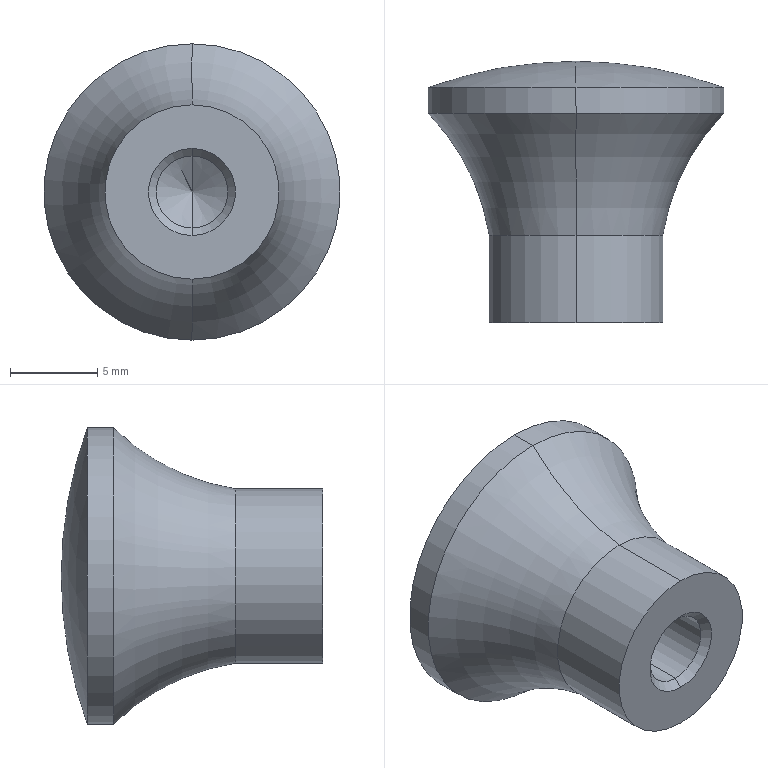Part | STEP file | HAQ07-M5^Air source cover plate | 1 solid | 15 faces | box 17 x 15 x 17 mm | volume 1673 mm3 | cylinder 6 | cone 4 | torus 2 | sphere 2 | plane 1 | commonest cylinder face diameters 4.134 x2 10 x2 17 x2
STEP:
#1=CARTESIAN_POINT('',(0.,0.,0.));
#2=DIRECTION('',(0.,0.,1.));
#3=DIRECTION('',(1.,0.,0.));
#4=AXIS2_PLACEMENT_3D('',#1,#2,#3);
#5=CARTESIAN_POINT('',(0.,18.75,-2.067));
#6=VERTEX_POINT('',#5);
#7=CARTESIAN_POINT('',(0.,18.75,2.067));
#8=VERTEX_POINT('',#7);
#9=CARTESIAN_POINT('',(0.,18.75,0.));
#10=DIRECTION('',(0.,1.,0.));
#11=DIRECTION('',(0.,0.,1.));
#12=AXIS2_PLACEMENT_3D('',#9,#10,#11);
#13=CIRCLE('',#12,2.067);
#14=CARTESIAN_POINT('',(0.,-480.057,0.));
#15=DIRECTION('',(0.,-1.,0.));
#16=DIRECTION('',(0.,0.,-1.));
#17=AXIS2_PLACEMENT_3D('',#14,#15,#16);
#18=CONICAL_SURFACE('',#17,866.025,1.047);
#19=CARTESIAN_POINT('',(9.425,-498.807));
#20=DIRECTION('',(-1.,0.));
#21=VECTOR('',#20,1.);
#22=LINE('',#19,#21);
#23=(GEOMETRIC_REPRESENTATION_CONTEXT(2)PARAMETRIC_REPRESENTATION_CONTEXT()REPRESENTATION_CONTEXT('',''));
#24=DEFINITIONAL_REPRESENTATION('',(#22),#23);
#25=PCURVE('',#18,#24);
#26=CARTESIAN_POINT('',(0.,19.943,0.));
#27=DIRECTION('',(0.,-1.,0.));
#28=DIRECTION('',(0.,0.,1.));
#29=AXIS2_PLACEMENT_3D('',#26,#27,#28);
#30=CYLINDRICAL_SURFACE('',#29,2.067);
#31=CARTESIAN_POINT('',(6.283,1.193));
#32=DIRECTION('',(-1.,0.));
#33=VECTOR('',#32,1.);
#34=LINE('',#31,#33);
#35=(GEOMETRIC_REPRESENTATION_CONTEXT(2)PARAMETRIC_REPRESENTATION_CONTEXT()REPRESENTATION_CONTEXT('',''));
#36=DEFINITIONAL_REPRESENTATION('',(#34),#35);
#37=PCURVE('',#30,#36);
#38=SURFACE_CURVE('',#13,(#25,#37),.PCURVE_S1.);
#39=EDGE_CURVE('',#6,#8,#38,.T.);
#40=ORIENTED_EDGE('',*,*,#39,.T.);
#41=CARTESIAN_POINT('',(0.,19.943,0.));
#42=VERTEX_POINT('',#41);
#43=CARTESIAN_POINT('',(0.,-480.057,866.025));
#44=DIRECTION('',(0.,-0.5,0.866));
#45=VECTOR('',#44,1.);
#46=LINE('',#43,#45);
#47=CARTESIAN_POINT('',(3.142,0.));
#48=DIRECTION('',(0.,1.));
#49=VECTOR('',#48,1.);
#50=LINE('',#47,#49);
#51=(GEOMETRIC_REPRESENTATION_CONTEXT(2)PARAMETRIC_REPRESENTATION_CONTEXT()REPRESENTATION_CONTEXT('',''));
#52=DEFINITIONAL_REPRESENTATION('',(#50),#51);
#53=PCURVE('',#18,#52);
#54=CARTESIAN_POINT('',(0.,-480.057,0.));
#55=DIRECTION('',(0.,-1.,0.));
#56=DIRECTION('',(0.,0.,-1.));
#57=AXIS2_PLACEMENT_3D('',#54,#55,#56);
#58=CONICAL_SURFACE('',#57,866.025,1.047);
#59=CARTESIAN_POINT('',(3.142,0.));
#60=DIRECTION('',(0.,1.));
#61=VECTOR('',#60,1.);
#62=LINE('',#59,#61);
#63=(GEOMETRIC_REPRESENTATION_CONTEXT(2)PARAMETRIC_REPRESENTATION_CONTEXT()REPRESENTATION_CONTEXT('',''));
#64=DEFINITIONAL_REPRESENTATION('',(#62),#63);
#65=PCURVE('',#58,#64);
#66=SURFACE_CURVE('',#46,(#53,#65),.PCURVE_S1.);
#67=EDGE_CURVE('',#42,#8,#66,.T.);
#68=ORIENTED_EDGE('',*,*,#67,.F.);
#69=CARTESIAN_POINT('',(0.,-480.057,-866.025));
#70=DIRECTION('',(0.,-0.5,-0.866));
#71=VECTOR('',#70,1.);
#72=LINE('',#69,#71);
#73=CARTESIAN_POINT('',(6.283,-500.));
#74=CARTESIAN_POINT('',(6.283,-499.982));
#75=CARTESIAN_POINT('',(6.283,-499.946));
#76=CARTESIAN_POINT('',(6.283,-499.892));
#77=CARTESIAN_POINT('',(6.283,-499.837));
#78=CARTESIAN_POINT('',(6.283,-499.783));
#79=CARTESIAN_POINT('',(6.283,-499.729));
#80=CARTESIAN_POINT('',(6.283,-499.675));
#81=CARTESIAN_POINT('',(6.283,-499.62));
#82=CARTESIAN_POINT('',(6.283,-499.566));
#83=CARTESIAN_POINT('',(6.283,-499.512));
#84=CARTESIAN_POINT('',(6.283,-499.458));
#85=CARTESIAN_POINT('',(6.283,-499.403));
#86=CARTESIAN_POINT('',(6.283,-499.349));
#87=CARTESIAN_POINT('',(6.283,-499.295));
#88=CARTESIAN_POINT('',(6.283,-499.241));
#89=CARTESIAN_POINT('',(6.283,-499.186));
#90=CARTESIAN_POINT('',(6.283,-499.132));
#91=CARTESIAN_POINT('',(6.283,-499.078));
#92=CARTESIAN_POINT('',(6.283,-499.024));
#93=CARTESIAN_POINT('',(6.283,-498.969));
#94=CARTESIAN_POINT('',(6.283,-498.915));
#95=CARTESIAN_POINT('',(6.283,-498.861));
#96=CARTESIAN_POINT('',(6.283,-498.825));
#97=CARTESIAN_POINT('',(6.283,-498.807));
#98=B_SPLINE_CURVE_WITH_KNOTS('',3,(#73,#74,#75,#76,#77,#78,#79,#80,#81,#82,#83,#84,#85,#86,#87,#88,#89,#90,#91,#92,#93,#94,#95,#96,#97),.UNSPECIFIED.,.F.,.F.,(4,1,1,1,1,1,1,1,1,1,1,1,1,1,1,1,1,1,1,1,1,1,4),(-1000.,-999.892,-999.783,-999.675,-999.566,-999.458,-999.349,-999.241,-999.132,-999.024,-998.915,-998.807,-998.698,-998.59,-998.481,-998.373,-998.264,-998.156,-998.047,-997.939,-997.83,-997.722,-997.613),.QUASI_UNIFORM_KNOTS.);
#99=(GEOMETRIC_REPRESENTATION_CONTEXT(2)PARAMETRIC_REPRESENTATION_CONTEXT()REPRESENTATION_CONTEXT('',''));
#100=DEFINITIONAL_REPRESENTATION('',(#98),#99);
#101=PCURVE('',#18,#100);
#102=CARTESIAN_POINT('',(0.,0.));
#103=DIRECTION('',(0.,1.));
#104=VECTOR('',#103,1.);
#105=LINE('',#102,#104);
#106=(GEOMETRIC_REPRESENTATION_CONTEXT(2)PARAMETRIC_REPRESENTATION_CONTEXT()REPRESENTATION_CONTEXT('',''));
#107=DEFINITIONAL_REPRESENTATION('',(#105),#106);
#108=PCURVE('',#58,#107);
#109=SURFACE_CURVE('',#72,(#101,#108),.PCURVE_S1.);
#110=EDGE_CURVE('',#42,#6,#109,.T.);
#111=ORIENTED_EDGE('',*,*,#110,.T.);
#112=EDGE_LOOP('',(#40,#68,#111));
#113=FACE_BOUND('',#112,.F.);
#114=ADVANCED_FACE('',(#113),#18,.F.);
#115=CARTESIAN_POINT('',(0.,10.433,2.067));
#116=VERTEX_POINT('',#115);
#117=CARTESIAN_POINT('',(0.,19.943,2.067));
#118=DIRECTION('',(0.,-1.,0.));
#119=VECTOR('',#118,1.);
#120=LINE('',#117,#119);
#121=CARTESIAN_POINT('',(0.,19.943,0.));
#122=DIRECTION('',(0.,-1.,0.));
#123=DIRECTION('',(0.,0.,1.));
#124=AXIS2_PLACEMENT_3D('',#121,#122,#123);
#125=CYLINDRICAL_SURFACE('',#124,2.067);
#126=CARTESIAN_POINT('',(6.283,0.));
#127=DIRECTION('',(0.,1.));
#128=VECTOR('',#127,1.);
#129=LINE('',#126,#128);
#130=(GEOMETRIC_REPRESENTATION_CONTEXT(2)PARAMETRIC_REPRESENTATION_CONTEXT()REPRESENTATION_CONTEXT('',''));
#131=DEFINITIONAL_REPRESENTATION('',(#129),#130);
#132=PCURVE('',#125,#131);
#133=CARTESIAN_POINT('',(0.,0.));
#134=DIRECTION('',(0.,1.));
#135=VECTOR('',#134,1.);
#136=LINE('',#133,#135);
#137=(GEOMETRIC_REPRESENTATION_CONTEXT(2)PARAMETRIC_REPRESENTATION_CONTEXT()REPRESENTATION_CONTEXT('',''));
#138=DEFINITIONAL_REPRESENTATION('',(#136),#137);
#139=PCURVE('',#30,#138);
#140=SURFACE_CURVE('',#120,(#132,#139),.PCURVE_S1.);
#141=EDGE_CURVE('',#8,#116,#140,.T.);
#142=ORIENTED_EDGE('',*,*,#141,.T.);
#143=CARTESIAN_POINT('',(0.,10.433,-2.067));
#144=VERTEX_POINT('',#143);
#145=CARTESIAN_POINT('',(0.,10.433,0.));
#146=DIRECTION('',(0.,1.,0.));
#147=DIRECTION('',(0.,0.,1.));
#148=AXIS2_PLACEMENT_3D('',#145,#146,#147);
#149=CIRCLE('',#148,2.067);
#150=CARTESIAN_POINT('',(6.283,9.51));
#151=DIRECTION('',(-1.,0.));
#152=VECTOR('',#151,1.);
#153=LINE('',#150,#152);
#154=(GEOMETRIC_REPRESENTATION_CONTEXT(2)PARAMETRIC_REPRESENTATION_CONTEXT()REPRESENTATION_CONTEXT('',''));
#155=DEFINITIONAL_REPRESENTATION('',(#153),#154);
#156=PCURVE('',#125,#155);
#157=CARTESIAN_POINT('',(0.,10.433,0.));
#158=DIRECTION('',(0.,-1.,0.));
#159=DIRECTION('',(0.,0.,-1.));
#160=AXIS2_PLACEMENT_3D('',#157,#158,#159);
#161=CONICAL_SURFACE('',#160,2.067,0.7854);
#162=CARTESIAN_POINT('',(3.142,0.));
#163=DIRECTION('',(-1.,0.));
#164=VECTOR('',#163,1.);
#165=LINE('',#162,#164);
#166=(GEOMETRIC_REPRESENTATION_CONTEXT(2)PARAMETRIC_REPRESENTATION_CONTEXT()REPRESENTATION_CONTEXT('',''));
#167=DEFINITIONAL_REPRESENTATION('',(#165),#166);
#168=PCURVE('',#161,#167);
#169=SURFACE_CURVE('',#149,(#156,#168),.PCURVE_S1.);
#170=EDGE_CURVE('',#116,#144,#169,.T.);
#171=ORIENTED_EDGE('',*,*,#170,.T.);
#172=CARTESIAN_POINT('',(0.,19.943,-2.067));
#173=DIRECTION('',(0.,-1.,0.));
#174=VECTOR('',#173,1.);
#175=LINE('',#172,#174);
#176=CARTESIAN_POINT('',(3.142,0.));
#177=DIRECTION('',(0.,1.));
#178=VECTOR('',#177,1.);
#179=LINE('',#176,#178);
#180=(GEOMETRIC_REPRESENTATION_CONTEXT(2)PARAMETRIC_REPRESENTATION_CONTEXT()REPRESENTATION_CONTEXT('',''));
#181=DEFINITIONAL_REPRESENTATION('',(#179),#180);
#182=PCURVE('',#125,#181);
#183=CARTESIAN_POINT('',(3.142,0.));
#184=DIRECTION('',(0.,1.));
#185=VECTOR('',#184,1.);
#186=LINE('',#183,#185);
#187=(GEOMETRIC_REPRESENTATION_CONTEXT(2)PARAMETRIC_REPRESENTATION_CONTEXT()REPRESENTATION_CONTEXT('',''));
#188=DEFINITIONAL_REPRESENTATION('',(#186),#187);
#189=PCURVE('',#30,#188);
#190=SURFACE_CURVE('',#175,(#182,#189),.PCURVE_S1.);
#191=EDGE_CURVE('',#6,#144,#190,.T.);
#192=ORIENTED_EDGE('',*,*,#191,.F.);
#193=CARTESIAN_POINT('',(0.,18.75,0.));
#194=DIRECTION('',(0.,1.,0.));
#195=DIRECTION('',(0.,0.,1.));
#196=AXIS2_PLACEMENT_3D('',#193,#194,#195);
#197=CIRCLE('',#196,2.067);
#198=CARTESIAN_POINT('',(6.283,1.193));
#199=DIRECTION('',(-1.,0.));
#200=VECTOR('',#199,1.);
#201=LINE('',#198,#200);
#202=(GEOMETRIC_REPRESENTATION_CONTEXT(2)PARAMETRIC_REPRESENTATION_CONTEXT()REPRESENTATION_CONTEXT('',''));
#203=DEFINITIONAL_REPRESENTATION('',(#201),#202);
#204=PCURVE('',#125,#203);
#205=CARTESIAN_POINT('',(3.142,-498.807));
#206=DIRECTION('',(-1.,0.));
#207=VECTOR('',#206,1.);
#208=LINE('',#205,#207);
#209=(GEOMETRIC_REPRESENTATION_CONTEXT(2)PARAMETRIC_REPRESENTATION_CONTEXT()REPRESENTATION_CONTEXT('',''));
#210=DEFINITIONAL_REPRESENTATION('',(#208),#209);
#211=PCURVE('',#58,#210);
#212=SURFACE_CURVE('',#197,(#204,#211),.PCURVE_S1.);
#213=EDGE_CURVE('',#8,#6,#212,.T.);
#214=ORIENTED_EDGE('',*,*,#213,.F.);
#215=EDGE_LOOP('',(#142,#171,#192,#214));
#216=FACE_BOUND('',#215,.F.);
#217=ADVANCED_FACE('',(#216),#125,.F.);
#218=CARTESIAN_POINT('',(0.,10.,-2.5));
#219=VERTEX_POINT('',#218);
#220=CARTESIAN_POINT('',(0.,10.433,-2.067));
#221=DIRECTION('',(0.,-0.7071,-0.7071));
#222=VECTOR('',#221,1.);
#223=LINE('',#220,#222);
#224=CARTESIAN_POINT('',(0.,10.433,0.));
#225=DIRECTION('',(0.,-1.,0.));
#226=DIRECTION('',(0.,0.,-1.));
#227=AXIS2_PLACEMENT_3D('',#224,#225,#226);
#228=CONICAL_SURFACE('',#227,2.067,0.7854);
#229=CARTESIAN_POINT('',(6.283,0.));
#230=DIRECTION('',(0.,1.));
#231=VECTOR('',#230,1.);
#232=LINE('',#229,#231);
#233=(GEOMETRIC_REPRESENTATION_CONTEXT(2)PARAMETRIC_REPRESENTATION_CONTEXT()REPRESENTATION_CONTEXT('',''));
#234=DEFINITIONAL_REPRESENTATION('',(#232),#233);
#235=PCURVE('',#228,#234);
#236=CARTESIAN_POINT('',(0.,0.));
#237=DIRECTION('',(0.,1.));
#238=VECTOR('',#237,1.);
#239=LINE('',#236,#238);
#240=(GEOMETRIC_REPRESENTATION_CONTEXT(2)PARAMETRIC_REPRESENTATION_CONTEXT()REPRESENTATION_CONTEXT('',''));
#241=DEFINITIONAL_REPRESENTATION('',(#239),#240);
#242=PCURVE('',#161,#241);
#243=SURFACE_CURVE('',#223,(#235,#242),.PCURVE_S1.);
#244=EDGE_CURVE('',#144,#219,#243,.T.);
#245=ORIENTED_EDGE('',*,*,#244,.T.);
#246=CARTESIAN_POINT('',(0.,10.,2.5));
#247=VERTEX_POINT('',#246);
#248=CARTESIAN_POINT('',(0.,10.,0.));
#249=DIRECTION('',(0.,1.,0.));
#250=DIRECTION('',(0.,0.,1.));
#251=AXIS2_PLACEMENT_3D('',#248,#249,#250);
#252=CIRCLE('',#251,2.5);
#253=CARTESIAN_POINT('',(9.425,0.433));
#254=DIRECTION('',(-1.,0.));
#255=VECTOR('',#254,1.);
#256=LINE('',#253,#255);
#257=(GEOMETRIC_REPRESENTATION_CONTEXT(2)PARAMETRIC_REPRESENTATION_CONTEXT()REPRESENTATION_CONTEXT('',''));
#258=DEFINITIONAL_REPRESENTATION('',(#256),#257);
#259=PCURVE('',#228,#258);
#260=CARTESIAN_POINT('',(0.,10.,2.5));
#261=DIRECTION('',(0.,1.,0.));
#262=DIRECTION('',(1.,0.,0.));
#263=AXIS2_PLACEMENT_3D('',#260,#261,#262);
#264=PLANE('',#263);
#265=CARTESIAN_POINT('',(0.,2.5));
#266=DIRECTION('',(0.,-1.));
#267=AXIS2_PLACEMENT_2D('',#265,#266);
#268=CIRCLE('',#267,2.5);
#269=(GEOMETRIC_REPRESENTATION_CONTEXT(2)PARAMETRIC_REPRESENTATION_CONTEXT()REPRESENTATION_CONTEXT('',''));
#270=DEFINITIONAL_REPRESENTATION('',(#268),#269);
#271=PCURVE('',#264,#270);
#272=SURFACE_CURVE('',#252,(#259,#271),.PCURVE_S1.);
#273=EDGE_CURVE('',#219,#247,#272,.T.);
#274=ORIENTED_EDGE('',*,*,#273,.T.);
#275=CARTESIAN_POINT('',(0.,10.433,2.067));
#276=DIRECTION('',(0.,-0.7071,0.7071));
#277=VECTOR('',#276,1.);
#278=LINE('',#275,#277);
#279=CARTESIAN_POINT('',(3.142,0.));
#280=DIRECTION('',(0.,1.));
#281=VECTOR('',#280,1.);
#282=LINE('',#279,#281);
#283=(GEOMETRIC_REPRESENTATION_CONTEXT(2)PARAMETRIC_REPRESENTATION_CONTEXT()REPRESENTATION_CONTEXT('',''));
#284=DEFINITIONAL_REPRESENTATION('',(#282),#283);
#285=PCURVE('',#228,#284);
#286=CARTESIAN_POINT('',(3.142,0.));
#287=DIRECTION('',(0.,1.));
#288=VECTOR('',#287,1.);
#289=LINE('',#286,#288);
#290=(GEOMETRIC_REPRESENTATION_CONTEXT(2)PARAMETRIC_REPRESENTATION_CONTEXT()REPRESENTATION_CONTEXT('',''));
#291=DEFINITIONAL_REPRESENTATION('',(#289),#290);
#292=PCURVE('',#161,#291);
#293=SURFACE_CURVE('',#278,(#285,#292),.PCURVE_S1.);
#294=EDGE_CURVE('',#116,#247,#293,.T.);
#295=ORIENTED_EDGE('',*,*,#294,.F.);
#296=CARTESIAN_POINT('',(0.,10.433,0.));
#297=DIRECTION('',(0.,1.,0.));
#298=DIRECTION('',(0.,0.,1.));
#299=AXIS2_PLACEMENT_3D('',#296,#297,#298);
#300=CIRCLE('',#299,2.067);
#301=CARTESIAN_POINT('',(9.425,0.));
#302=DIRECTION('',(-1.,0.));
#303=VECTOR('',#302,1.);
#304=LINE('',#301,#303);
#305=(GEOMETRIC_REPRESENTATION_CONTEXT(2)PARAMETRIC_REPRESENTATION_CONTEXT()REPRESENTATION_CONTEXT('',''));
#306=DEFINITIONAL_REPRESENTATION('',(#304),#305);
#307=PCURVE('',#228,#306);
#308=CARTESIAN_POINT('',(6.283,9.51));
#309=DIRECTION('',(-1.,0.));
#310=VECTOR('',#309,1.);
#311=LINE('',#308,#310);
#312=(GEOMETRIC_REPRESENTATION_CONTEXT(2)PARAMETRIC_REPRESENTATION_CONTEXT()REPRESENTATION_CONTEXT('',''));
#313=DEFINITIONAL_REPRESENTATION('',(#311),#312);
#314=PCURVE('',#30,#313);
#315=SURFACE_CURVE('',#300,(#307,#314),.PCURVE_S1.);
#316=EDGE_CURVE('',#144,#116,#315,.T.);
#317=ORIENTED_EDGE('',*,*,#316,.F.);
#318=EDGE_LOOP('',(#245,#274,#295,#317));
#319=FACE_BOUND('',#318,.F.);
#320=ADVANCED_FACE('',(#319),#228,.F.);
#321=CARTESIAN_POINT('',(0.,15.,-5.));
#322=VERTEX_POINT('',#321);
#323=CARTESIAN_POINT('',(0.,15.,5.));
#324=VERTEX_POINT('',#323);
#325=CARTESIAN_POINT('',(0.,15.,0.));
#326=DIRECTION('',(0.,1.,0.));
#327=DIRECTION('',(0.,0.,1.));
#328=AXIS2_PLACEMENT_3D('',#325,#326,#327);
#329=CIRCLE('',#328,5.);
#330=CARTESIAN_POINT('',(0.,19.943,0.));
#331=DIRECTION('',(0.,-1.,0.));
#332=DIRECTION('',(0.,0.,1.));
#333=AXIS2_PLACEMENT_3D('',#330,#331,#332);
#334=CYLINDRICAL_SURFACE('',#333,5.);
#335=CARTESIAN_POINT('',(6.283,4.943));
#336=DIRECTION('',(-1.,0.));
#337=VECTOR('',#336,1.);
#338=LINE('',#335,#337);
#339=(GEOMETRIC_REPRESENTATION_CONTEXT(2)PARAMETRIC_REPRESENTATION_CONTEXT()REPRESENTATION_CONTEXT('',''));
#340=DEFINITIONAL_REPRESENTATION('',(#338),#339);
#341=PCURVE('',#334,#340);
#342=CARTESIAN_POINT('',(0.,13.073,0.));
#343=DIRECTION('',(0.,1.,0.));
#344=DIRECTION('',(0.,0.,1.));
#345=AXIS2_PLACEMENT_3D('',#342,#343,#344);
#346=TOROIDAL_SURFACE('',#345,17.604,12.75);
#347=CARTESIAN_POINT('',(0.,2.99));
#348=DIRECTION('',(1.,0.));
#349=VECTOR('',#348,1.);
#350=LINE('',#347,#349);
#351=(GEOMETRIC_REPRESENTATION_CONTEXT(2)PARAMETRIC_REPRESENTATION_CONTEXT()REPRESENTATION_CONTEXT('',''));
#352=DEFINITIONAL_REPRESENTATION('',(#350),#351);
#353=PCURVE('',#346,#352);
#354=SURFACE_CURVE('',#329,(#341,#353),.PCURVE_S1.);
#355=EDGE_CURVE('',#322,#324,#354,.T.);
#356=ORIENTED_EDGE('',*,*,#355,.F.);
#357=CARTESIAN_POINT('',(0.,10.,-5.));
#358=VERTEX_POINT('',#357);
#359=CARTESIAN_POINT('',(0.,19.943,-5.));
#360=DIRECTION('',(0.,-1.,0.));
#361=VECTOR('',#360,1.);
#362=LINE('',#359,#361);
#363=CARTESIAN_POINT('',(3.142,0.));
#364=DIRECTION('',(0.,1.));
#365=VECTOR('',#364,1.);
#366=LINE('',#363,#365);
#367=(GEOMETRIC_REPRESENTATION_CONTEXT(2)PARAMETRIC_REPRESENTATION_CONTEXT()REPRESENTATION_CONTEXT('',''));
#368=DEFINITIONAL_REPRESENTATION('',(#366),#367);
#369=PCURVE('',#334,#368);
#370=CARTESIAN_POINT('',(0.,19.943,0.));
#371=DIRECTION('',(0.,-1.,0.));
#372=DIRECTION('',(0.,0.,1.));
#373=AXIS2_PLACEMENT_3D('',#370,#371,#372);
#374=CYLINDRICAL_SURFACE('',#373,5.);
#375=CARTESIAN_POINT('',(3.142,0.));
#376=DIRECTION('',(0.,1.));
#377=VECTOR('',#376,1.);
#378=LINE('',#375,#377);
#379=(GEOMETRIC_REPRESENTATION_CONTEXT(2)PARAMETRIC_REPRESENTATION_CONTEXT()REPRESENTATION_CONTEXT('',''));
#380=DEFINITIONAL_REPRESENTATION('',(#378),#379);
#381=PCURVE('',#374,#380);
#382=SURFACE_CURVE('',#362,(#369,#381),.PCURVE_S1.);
#383=EDGE_CURVE('',#322,#358,#382,.T.);
#384=ORIENTED_EDGE('',*,*,#383,.T.);
#385=CARTESIAN_POINT('',(0.,10.,5.));
#386=VERTEX_POINT('',#385);
#387=CARTESIAN_POINT('',(0.,10.,0.));
#388=DIRECTION('',(0.,1.,0.));
#389=DIRECTION('',(0.,0.,1.));
#390=AXIS2_PLACEMENT_3D('',#387,#388,#389);
#391=CIRCLE('',#390,5.);
#392=CARTESIAN_POINT('',(6.283,9.943));
#393=DIRECTION('',(-1.,0.));
#394=VECTOR('',#393,1.);
#395=LINE('',#392,#394);
#396=(GEOMETRIC_REPRESENTATION_CONTEXT(2)PARAMETRIC_REPRESENTATION_CONTEXT()REPRESENTATION_CONTEXT('',''));
#397=DEFINITIONAL_REPRESENTATION('',(#395),#396);
#398=PCURVE('',#334,#397);
#399=CARTESIAN_POINT('',(0.,2.5));
#400=DIRECTION('',(0.,-1.));
#401=AXIS2_PLACEMENT_2D('',#399,#400);
#402=CIRCLE('',#401,5.);
#403=(GEOMETRIC_REPRESENTATION_CONTEXT(2)PARAMETRIC_REPRESENTATION_CONTEXT()REPRESENTATION_CONTEXT('',''));
#404=DEFINITIONAL_REPRESENTATION('',(#402),#403);
#405=PCURVE('',#264,#404);
#406=SURFACE_CURVE('',#391,(#398,#405),.PCURVE_S1.);
#407=EDGE_CURVE('',#358,#386,#406,.T.);
#408=ORIENTED_EDGE('',*,*,#407,.T.);
#409=CARTESIAN_POINT('',(0.,19.943,5.));
#410=DIRECTION('',(0.,-1.,0.));
#411=VECTOR('',#410,1.);
#412=LINE('',#409,#411);
#413=CARTESIAN_POINT('',(0.,0.));
#414=DIRECTION('',(0.,1.));
#415=VECTOR('',#414,1.);
#416=LINE('',#413,#415);
#417=(GEOMETRIC_REPRESENTATION_CONTEXT(2)PARAMETRIC_REPRESENTATION_CONTEXT()REPRESENTATION_CONTEXT('',''));
#418=DEFINITIONAL_REPRESENTATION('',(#416),#417);
#419=PCURVE('',#334,#418);
#420=CARTESIAN_POINT('',(6.283,0.));
#421=DIRECTION('',(0.,1.));
#422=VECTOR('',#421,1.);
#423=LINE('',#420,#422);
#424=(GEOMETRIC_REPRESENTATION_CONTEXT(2)PARAMETRIC_REPRESENTATION_CONTEXT()REPRESENTATION_CONTEXT('',''));
#425=DEFINITIONAL_REPRESENTATION('',(#423),#424);
#426=PCURVE('',#374,#425);
#427=SURFACE_CURVE('',#412,(#419,#426),.PCURVE_S1.);
#428=EDGE_CURVE('',#324,#386,#427,.T.);
#429=ORIENTED_EDGE('',*,*,#428,.F.);
#430=EDGE_LOOP('',(#356,#384,#408,#429));
#431=FACE_BOUND('',#430,.T.);
#432=ADVANCED_FACE('',(#431),#334,.T.);
#433=CARTESIAN_POINT('',(0.,22.,8.5));
#434=VERTEX_POINT('',#433);
#435=CARTESIAN_POINT('',(0.,13.073,17.604));
#436=DIRECTION('',(-1.,0.,0.));
#437=DIRECTION('',(0.,-1.,0.));
#438=AXIS2_PLACEMENT_3D('',#435,#436,#437);
#439=CIRCLE('',#438,12.75);
#440=CARTESIAN_POINT('',(6.283,-1.571));
#441=DIRECTION('',(0.,1.));
#442=VECTOR('',#441,1.);
#443=LINE('',#440,#442);
#444=(GEOMETRIC_REPRESENTATION_CONTEXT(2)PARAMETRIC_REPRESENTATION_CONTEXT()REPRESENTATION_CONTEXT('',''));
#445=DEFINITIONAL_REPRESENTATION('',(#443),#444);
#446=PCURVE('',#346,#445);
#447=CARTESIAN_POINT('',(0.,13.073,0.));
#448=DIRECTION('',(0.,1.,0.));
#449=DIRECTION('',(0.,0.,1.));
#450=AXIS2_PLACEMENT_3D('',#447,#448,#449);
#451=TOROIDAL_SURFACE('',#450,17.604,12.75);
#452=CARTESIAN_POINT('',(0.,-1.571));
#453=DIRECTION('',(0.,1.));
#454=VECTOR('',#453,1.);
#455=LINE('',#452,#454);
#456=(GEOMETRIC_REPRESENTATION_CONTEXT(2)PARAMETRIC_REPRESENTATION_CONTEXT()REPRESENTATION_CONTEXT('',''));
#457=DEFINITIONAL_REPRESENTATION('',(#455),#456);
#458=PCURVE('',#451,#457);
#459=SURFACE_CURVE('',#439,(#446,#458),.PCURVE_S1.);
#460=EDGE_CURVE('',#434,#324,#459,.T.);
#461=ORIENTED_EDGE('',*,*,#460,.T.);
#462=ORIENTED_EDGE('',*,*,#355,.F.);
#463=CARTESIAN_POINT('',(0.,22.,-8.5));
#464=VERTEX_POINT('',#463);
#465=CARTESIAN_POINT('',(0.,13.073,-17.604));
#466=DIRECTION('',(1.,0.,0.));
#467=DIRECTION('',(0.,1.,0.));
#468=AXIS2_PLACEMENT_3D('',#465,#466,#467);
#469=CIRCLE('',#468,12.75);
#470=CARTESIAN_POINT('',(3.142,1.571));
#471=DIRECTION('',(0.,1.));
#472=VECTOR('',#471,1.);
#473=LINE('',#470,#472);
#474=(GEOMETRIC_REPRESENTATION_CONTEXT(2)PARAMETRIC_REPRESENTATION_CONTEXT()REPRESENTATION_CONTEXT('',''));
#475=DEFINITIONAL_REPRESENTATION('',(#473),#474);
#476=PCURVE('',#346,#475);
#477=CARTESIAN_POINT('',(3.142,1.571));
#478=DIRECTION('',(0.,1.));
#479=VECTOR('',#478,1.);
#480=LINE('',#477,#479);
#481=(GEOMETRIC_REPRESENTATION_CONTEXT(2)PARAMETRIC_REPRESENTATION_CONTEXT()REPRESENTATION_CONTEXT('',''));
#482=DEFINITIONAL_REPRESENTATION('',(#480),#481);
#483=PCURVE('',#451,#482);
#484=SURFACE_CURVE('',#469,(#476,#483),.PCURVE_S1.);
#485=EDGE_CURVE('',#464,#322,#484,.T.);
#486=ORIENTED_EDGE('',*,*,#485,.F.);
#487=CARTESIAN_POINT('',(0.,22.,0.));
#488=DIRECTION('',(0.,1.,0.));
#489=DIRECTION('',(0.,0.,1.));
#490=AXIS2_PLACEMENT_3D('',#487,#488,#489);
#491=CIRCLE('',#490,8.5);
#492=CARTESIAN_POINT('',(0.,2.366));
#493=DIRECTION('',(1.,0.));
#494=VECTOR('',#493,1.);
#495=LINE('',#492,#494);
#496=(GEOMETRIC_REPRESENTATION_CONTEXT(2)PARAMETRIC_REPRESENTATION_CONTEXT()REPRESENTATION_CONTEXT('',''));
#497=DEFINITIONAL_REPRESENTATION('',(#495),#496);
#498=PCURVE('',#346,#497);
#499=CARTESIAN_POINT('',(0.,19.943,0.));
#500=DIRECTION('',(0.,-1.,0.));
#501=DIRECTION('',(0.,0.,1.));
#502=AXIS2_PLACEMENT_3D('',#499,#500,#501);
#503=CYLINDRICAL_SURFACE('',#502,8.5);
#504=CARTESIAN_POINT('',(6.283,-2.057));
#505=DIRECTION('',(-1.,0.));
#506=VECTOR('',#505,1.);
#507=LINE('',#504,#506);
#508=(GEOMETRIC_REPRESENTATION_CONTEXT(2)PARAMETRIC_REPRESENTATION_CONTEXT()REPRESENTATION_CONTEXT('',''));
#509=DEFINITIONAL_REPRESENTATION('',(#507),#508);
#510=PCURVE('',#503,#509);
#511=SURFACE_CURVE('',#491,(#498,#510),.PCURVE_S1.);
#512=EDGE_CURVE('',#464,#434,#511,.T.);
#513=ORIENTED_EDGE('',*,*,#512,.T.);
#514=EDGE_LOOP('',(#461,#462,#486,#513));
#515=FACE_BOUND('',#514,.F.);
#516=ADVANCED_FACE('',(#515),#346,.F.);
#517=CARTESIAN_POINT('',(0.,23.5,-8.5));
#518=VERTEX_POINT('',#517);
#519=CARTESIAN_POINT('',(0.,23.5,8.5));
#520=VERTEX_POINT('',#519);
#521=CARTESIAN_POINT('',(0.,23.5,0.));
#522=DIRECTION('',(0.,1.,0.));
#523=DIRECTION('',(0.,0.,1.));
#524=AXIS2_PLACEMENT_3D('',#521,#522,#523);
#525=CIRCLE('',#524,8.5);
#526=CARTESIAN_POINT('',(6.283,-3.557));
#527=DIRECTION('',(-1.,0.));
#528=VECTOR('',#527,1.);
#529=LINE('',#526,#528);
#530=(GEOMETRIC_REPRESENTATION_CONTEXT(2)PARAMETRIC_REPRESENTATION_CONTEXT()REPRESENTATION_CONTEXT('',''));
#531=DEFINITIONAL_REPRESENTATION('',(#529),#530);
#532=PCURVE('',#503,#531);
#533=CARTESIAN_POINT('',(0.,0.1667,0.));
#534=DIRECTION('',(-1.,0.,0.));
#535=DIRECTION('',(0.,0.,-1.));
#536=AXIS2_PLACEMENT_3D('',#533,#534,#535);
#537=SPHERICAL_SURFACE('',#536,24.833);
#538=CARTESIAN_POINT('',(5.062,0.));
#539=CARTESIAN_POINT('',(5.062,0.01629));
#540=CARTESIAN_POINT('',(5.06,0.04888));
#541=CARTESIAN_POINT('',(5.05,0.09688));
#542=CARTESIAN_POINT('',(5.033,0.1431));
#543=CARTESIAN_POINT('',(5.011,0.1867));
#544=CARTESIAN_POINT('',(4.982,0.2268));
#545=CARTESIAN_POINT('',(4.947,0.2625));
#546=CARTESIAN_POINT('',(4.908,0.2931));
#547=CARTESIAN_POINT('',(4.863,0.3177));
#548=CARTESIAN_POINT('',(4.815,0.3358));
#549=CARTESIAN_POINT('',(4.764,0.3469));
#550=CARTESIAN_POINT('',(4.712,0.3506));
#551=CARTESIAN_POINT('',(4.66,0.3469));
#552=CARTESIAN_POINT('',(4.61,0.3358));
#553=CARTESIAN_POINT('',(4.562,0.3177));
#554=CARTESIAN_POINT('',(4.517,0.2931));
#555=CARTESIAN_POINT('',(4.477,0.2625));
#556=CARTESIAN_POINT('',(4.443,0.2268));
#557=CARTESIAN_POINT('',(4.414,0.1867));
#558=CARTESIAN_POINT('',(4.391,0.1431));
#559=CARTESIAN_POINT('',(4.375,0.09688));
#560=CARTESIAN_POINT('',(4.365,0.04888));
#561=CARTESIAN_POINT('',(4.363,0.01629));
#562=CARTESIAN_POINT('',(4.363,0.));
#563=B_SPLINE_CURVE_WITH_KNOTS('',3,(#538,#539,#540,#541,#542,#543,#544,#545,#546,#547,#548,#549,#550,#551,#552,#553,#554,#555,#556,#557,#558,#559,#560,#561,#562),.UNSPECIFIED.,.F.,.F.,(4,1,1,1,1,1,1,1,1,1,1,1,1,1,1,1,1,1,1,1,1,1,4),(3.142,3.284,3.427,3.57,3.713,3.856,3.998,4.141,4.284,4.427,4.57,4.712,4.855,4.998,5.141,5.284,5.426,5.569,5.712,5.855,5.998,6.14,6.283),.QUASI_UNIFORM_KNOTS.);
#564=(GEOMETRIC_REPRESENTATION_CONTEXT(2)PARAMETRIC_REPRESENTATION_CONTEXT()REPRESENTATION_CONTEXT('',''));
#565=DEFINITIONAL_REPRESENTATION('',(#563),#564);
#566=PCURVE('',#537,#565);
#567=SURFACE_CURVE('',#525,(#532,#566),.PCURVE_S1.);
#568=EDGE_CURVE('',#518,#520,#567,.T.);
#569=ORIENTED_EDGE('',*,*,#568,.F.);
#570=CARTESIAN_POINT('',(0.,19.943,-8.5));
#571=DIRECTION('',(0.,-1.,0.));
#572=VECTOR('',#571,1.);
#573=LINE('',#570,#572);
#574=CARTESIAN_POINT('',(3.142,0.));
#575=DIRECTION('',(0.,1.));
#576=VECTOR('',#575,1.);
#577=LINE('',#574,#576);
#578=(GEOMETRIC_REPRESENTATION_CONTEXT(2)PARAMETRIC_REPRESENTATION_CONTEXT()REPRESENTATION_CONTEXT('',''));
#579=DEFINITIONAL_REPRESENTATION('',(#577),#578);
#580=PCURVE('',#503,#579);
#581=CARTESIAN_POINT('',(0.,19.943,0.));
#582=DIRECTION('',(0.,-1.,0.));
#583=DIRECTION('',(0.,0.,1.));
#584=AXIS2_PLACEMENT_3D('',#581,#582,#583);
#585=CYLINDRICAL_SURFACE('',#584,8.5);
#586=CARTESIAN_POINT('',(3.142,0.));
#587=DIRECTION('',(0.,1.));
#588=VECTOR('',#587,1.);
#589=LINE('',#586,#588);
#590=(GEOMETRIC_REPRESENTATION_CONTEXT(2)PARAMETRIC_REPRESENTATION_CONTEXT()REPRESENTATION_CONTEXT('',''));
#591=DEFINITIONAL_REPRESENTATION('',(#589),#590);
#592=PCURVE('',#585,#591);
#593=SURFACE_CURVE('',#573,(#580,#592),.PCURVE_S1.);
#594=EDGE_CURVE('',#518,#464,#593,.T.);
#595=ORIENTED_EDGE('',*,*,#594,.T.);
#596=ORIENTED_EDGE('',*,*,#512,.T.);
#597=CARTESIAN_POINT('',(0.,19.943,8.5));
#598=DIRECTION('',(0.,-1.,0.));
#599=VECTOR('',#598,1.);
#600=LINE('',#597,#599);
#601=CARTESIAN_POINT('',(0.,0.));
#602=DIRECTION('',(0.,1.));
#603=VECTOR('',#602,1.);
#604=LINE('',#601,#603);
#605=(GEOMETRIC_REPRESENTATION_CONTEXT(2)PARAMETRIC_REPRESENTATION_CONTEXT()REPRESENTATION_CONTEXT('',''));
#606=DEFINITIONAL_REPRESENTATION('',(#604),#605);
#607=PCURVE('',#503,#606);
#608=CARTESIAN_POINT('',(6.283,0.));
#609=DIRECTION('',(0.,1.));
#610=VECTOR('',#609,1.);
#611=LINE('',#608,#610);
#612=(GEOMETRIC_REPRESENTATION_CONTEXT(2)PARAMETRIC_REPRESENTATION_CONTEXT()REPRESENTATION_CONTEXT('',''));
#613=DEFINITIONAL_REPRESENTATION('',(#611),#612);
#614=PCURVE('',#585,#613);
#615=SURFACE_CURVE('',#600,(#607,#614),.PCURVE_S1.);
#616=EDGE_CURVE('',#520,#434,#615,.T.);
#617=ORIENTED_EDGE('',*,*,#616,.F.);
#618=EDGE_LOOP('',(#569,#595,#596,#617));
#619=FACE_BOUND('',#618,.T.);
#620=ADVANCED_FACE('',(#619),#503,.T.);
#621=ORIENTED_EDGE('',*,*,#568,.T.);
#622=CARTESIAN_POINT('',(0.,25.,0.));
#623=VERTEX_POINT('',#622);
#624=CARTESIAN_POINT('',(0.,0.1667,0.));
#625=DIRECTION('',(-1.,0.,0.));
#626=DIRECTION('',(0.,-1.,0.));
#627=AXIS2_PLACEMENT_3D('',#624,#625,#626);
#628=CIRCLE('',#627,24.833);
#629=CARTESIAN_POINT('',(1.571,0.));
#630=DIRECTION('',(1.,0.));
#631=VECTOR('',#630,1.);
#632=LINE('',#629,#631);
#633=(GEOMETRIC_REPRESENTATION_CONTEXT(2)PARAMETRIC_REPRESENTATION_CONTEXT()REPRESENTATION_CONTEXT('',''));
#634=DEFINITIONAL_REPRESENTATION('',(#632),#633);
#635=PCURVE('',#537,#634);
#636=CARTESIAN_POINT('',(0.,0.1667,0.));
#637=DIRECTION('',(-1.,0.,0.));
#638=DIRECTION('',(0.,0.,-1.));
#639=AXIS2_PLACEMENT_3D('',#636,#637,#638);
#640=SPHERICAL_SURFACE('',#639,24.833);
#641=CARTESIAN_POINT('',(1.571,0.));
#642=DIRECTION('',(1.,0.));
#643=VECTOR('',#642,1.);
#644=LINE('',#641,#643);
#645=(GEOMETRIC_REPRESENTATION_CONTEXT(2)PARAMETRIC_REPRESENTATION_CONTEXT()REPRESENTATION_CONTEXT('',''));
#646=DEFINITIONAL_REPRESENTATION('',(#644),#645);
#647=PCURVE('',#640,#646);
#648=SURFACE_CURVE('',#628,(#635,#647),.PCURVE_S1.);
#649=EDGE_CURVE('',#520,#623,#648,.T.);
#650=ORIENTED_EDGE('',*,*,#649,.T.);
#651=CARTESIAN_POINT('',(0.,0.1667,0.));
#652=DIRECTION('',(1.,0.,0.));
#653=DIRECTION('',(0.,1.,0.));
#654=AXIS2_PLACEMENT_3D('',#651,#652,#653);
#655=CIRCLE('',#654,24.833);
#656=CARTESIAN_POINT('',(10.996,0.));
#657=DIRECTION('',(-1.,0.));
#658=VECTOR('',#657,1.);
#659=LINE('',#656,#658);
#660=(GEOMETRIC_REPRESENTATION_CONTEXT(2)PARAMETRIC_REPRESENTATION_CONTEXT()REPRESENTATION_CONTEXT('',''));
#661=DEFINITIONAL_REPRESENTATION('',(#659),#660);
#662=PCURVE('',#537,#661);
#663=CARTESIAN_POINT('',(10.996,0.));
#664=DIRECTION('',(-1.,0.));
#665=VECTOR('',#664,1.);
#666=LINE('',#663,#665);
#667=(GEOMETRIC_REPRESENTATION_CONTEXT(2)PARAMETRIC_REPRESENTATION_CONTEXT()REPRESENTATION_CONTEXT('',''));
#668=DEFINITIONAL_REPRESENTATION('',(#666),#667);
#669=PCURVE('',#640,#668);
#670=SURFACE_CURVE('',#655,(#662,#669),.PCURVE_S1.);
#671=EDGE_CURVE('',#518,#623,#670,.T.);
#672=ORIENTED_EDGE('',*,*,#671,.F.);
#673=EDGE_LOOP('',(#621,#650,#672));
#674=FACE_BOUND('',#673,.T.);
#675=ADVANCED_FACE('',(#674),#537,.T.);
#676=ORIENTED_EDGE('',*,*,#649,.F.);
#677=CARTESIAN_POINT('',(0.,23.5,0.));
#678=DIRECTION('',(0.,1.,0.));
#679=DIRECTION('',(0.,0.,1.));
#680=AXIS2_PLACEMENT_3D('',#677,#678,#679);
#681=CIRCLE('',#680,8.5);
#682=CARTESIAN_POINT('',(4.363,0.));
#683=CARTESIAN_POINT('',(4.363,-0.01629));
#684=CARTESIAN_POINT('',(4.365,-0.04888));
#685=CARTESIAN_POINT('',(4.375,-0.09688));
#686=CARTESIAN_POINT('',(4.391,-0.1431));
#687=CARTESIAN_POINT('',(4.414,-0.1867));
#688=CARTESIAN_POINT('',(4.443,-0.2268));
#689=CARTESIAN_POINT('',(4.477,-0.2625));
#690=CARTESIAN_POINT('',(4.517,-0.2931));
#691=CARTESIAN_POINT('',(4.562,-0.3177));
#692=CARTESIAN_POINT('',(4.61,-0.3358));
#693=CARTESIAN_POINT('',(4.66,-0.3469));
#694=CARTESIAN_POINT('',(4.712,-0.3506));
#695=CARTESIAN_POINT('',(4.764,-0.3469));
#696=CARTESIAN_POINT('',(4.815,-0.3358));
#697=CARTESIAN_POINT('',(4.863,-0.3177));
#698=CARTESIAN_POINT('',(4.908,-0.2931));
#699=CARTESIAN_POINT('',(4.947,-0.2625));
#700=CARTESIAN_POINT('',(4.982,-0.2268));
#701=CARTESIAN_POINT('',(5.011,-0.1867));
#702=CARTESIAN_POINT('',(5.033,-0.1431));
#703=CARTESIAN_POINT('',(5.05,-0.09688));
#704=CARTESIAN_POINT('',(5.06,-0.04888));
#705=CARTESIAN_POINT('',(5.062,-0.01629));
#706=CARTESIAN_POINT('',(5.062,0.));
#707=B_SPLINE_CURVE_WITH_KNOTS('',3,(#682,#683,#684,#685,#686,#687,#688,#689,#690,#691,#692,#693,#694,#695,#696,#697,#698,#699,#700,#701,#702,#703,#704,#705,#706),.UNSPECIFIED.,.F.,.F.,(4,1,1,1,1,1,1,1,1,1,1,1,1,1,1,1,1,1,1,1,1,1,4),(0.,0.1428,0.2856,0.4284,0.5712,0.714,0.8568,0.9996,1.142,1.285,1.428,1.571,1.714,1.856,1.999,2.142,2.285,2.428,2.57,2.713,2.856,2.999,3.142),.QUASI_UNIFORM_KNOTS.);
#708=(GEOMETRIC_REPRESENTATION_CONTEXT(2)PARAMETRIC_REPRESENTATION_CONTEXT()REPRESENTATION_CONTEXT('',''));
#709=DEFINITIONAL_REPRESENTATION('',(#707),#708);
#710=PCURVE('',#640,#709);
#711=CARTESIAN_POINT('',(6.283,-3.557));
#712=DIRECTION('',(-1.,0.));
#713=VECTOR('',#712,1.);
#714=LINE('',#711,#713);
#715=(GEOMETRIC_REPRESENTATION_CONTEXT(2)PARAMETRIC_REPRESENTATION_CONTEXT()REPRESENTATION_CONTEXT('',''));
#716=DEFINITIONAL_REPRESENTATION('',(#714),#715);
#717=PCURVE('',#585,#716);
#718=SURFACE_CURVE('',#681,(#710,#717),.PCURVE_S1.);
#719=EDGE_CURVE('',#520,#518,#718,.T.);
#720=ORIENTED_EDGE('',*,*,#719,.T.);
#721=ORIENTED_EDGE('',*,*,#671,.T.);
#722=EDGE_LOOP('',(#676,#720,#721));
#723=FACE_BOUND('',#722,.T.);
#724=ADVANCED_FACE('',(#723),#640,.T.);
#725=ORIENTED_EDGE('',*,*,#594,.F.);
#726=ORIENTED_EDGE('',*,*,#719,.F.);
#727=ORIENTED_EDGE('',*,*,#616,.T.);
#728=CARTESIAN_POINT('',(0.,22.,0.));
#729=DIRECTION('',(0.,1.,0.));
#730=DIRECTION('',(0.,0.,1.));
#731=AXIS2_PLACEMENT_3D('',#728,#729,#730);
#732=CIRCLE('',#731,8.5);
#733=CARTESIAN_POINT('',(6.283,-2.057));
#734=DIRECTION('',(-1.,0.));
#735=VECTOR('',#734,1.);
#736=LINE('',#733,#735);
#737=(GEOMETRIC_REPRESENTATION_CONTEXT(2)PARAMETRIC_REPRESENTATION_CONTEXT()REPRESENTATION_CONTEXT('',''));
#738=DEFINITIONAL_REPRESENTATION('',(#736),#737);
#739=PCURVE('',#585,#738);
#740=CARTESIAN_POINT('',(0.,2.366));
#741=DIRECTION('',(1.,0.));
#742=VECTOR('',#741,1.);
#743=LINE('',#740,#742);
#744=(GEOMETRIC_REPRESENTATION_CONTEXT(2)PARAMETRIC_REPRESENTATION_CONTEXT()REPRESENTATION_CONTEXT('',''));
#745=DEFINITIONAL_REPRESENTATION('',(#743),#744);
#746=PCURVE('',#451,#745);
#747=SURFACE_CURVE('',#732,(#739,#746),.PCURVE_S1.);
#748=EDGE_CURVE('',#434,#464,#747,.T.);
#749=ORIENTED_EDGE('',*,*,#748,.T.);
#750=EDGE_LOOP('',(#725,#726,#727,#749));
#751=FACE_BOUND('',#750,.T.);
#752=ADVANCED_FACE('',(#751),#585,.T.);
#753=CARTESIAN_POINT('',(0.,15.,0.));
#754=DIRECTION('',(0.,1.,0.));
#755=DIRECTION('',(0.,0.,1.));
#756=AXIS2_PLACEMENT_3D('',#753,#754,#755);
#757=CIRCLE('',#756,5.);
#758=CARTESIAN_POINT('',(0.,2.99));
#759=DIRECTION('',(1.,0.));
#760=VECTOR('',#759,1.);
#761=LINE('',#758,#760);
#762=(GEOMETRIC_REPRESENTATION_CONTEXT(2)PARAMETRIC_REPRESENTATION_CONTEXT()REPRESENTATION_CONTEXT('',''));
#763=DEFINITIONAL_REPRESENTATION('',(#761),#762);
#764=PCURVE('',#451,#763);
#765=CARTESIAN_POINT('',(6.283,4.943));
#766=DIRECTION('',(-1.,0.));
#767=VECTOR('',#766,1.);
#768=LINE('',#765,#767);
#769=(GEOMETRIC_REPRESENTATION_CONTEXT(2)PARAMETRIC_REPRESENTATION_CONTEXT()REPRESENTATION_CONTEXT('',''));
#770=DEFINITIONAL_REPRESENTATION('',(#768),#769);
#771=PCURVE('',#374,#770);
#772=SURFACE_CURVE('',#757,(#764,#771),.PCURVE_S1.);
#773=EDGE_CURVE('',#324,#322,#772,.T.);
#774=ORIENTED_EDGE('',*,*,#773,.F.);
#775=ORIENTED_EDGE('',*,*,#460,.F.);
#776=ORIENTED_EDGE('',*,*,#748,.T.);
#777=ORIENTED_EDGE('',*,*,#485,.T.);
#778=EDGE_LOOP('',(#774,#775,#776,#777));
#779=FACE_BOUND('',#778,.F.);
#780=ADVANCED_FACE('',(#779),#451,.F.);
#781=ORIENTED_EDGE('',*,*,#383,.F.);
#782=ORIENTED_EDGE('',*,*,#773,.F.);
#783=ORIENTED_EDGE('',*,*,#428,.T.);
#784=CARTESIAN_POINT('',(0.,10.,0.));
#785=DIRECTION('',(0.,1.,0.));
#786=DIRECTION('',(0.,0.,1.));
#787=AXIS2_PLACEMENT_3D('',#784,#785,#786);
#788=CIRCLE('',#787,5.);
#789=CARTESIAN_POINT('',(6.283,9.943));
#790=DIRECTION('',(-1.,0.));
#791=VECTOR('',#790,1.);
#792=LINE('',#789,#791);
#793=(GEOMETRIC_REPRESENTATION_CONTEXT(2)PARAMETRIC_REPRESENTATION_CONTEXT()REPRESENTATION_CONTEXT('',''));
#794=DEFINITIONAL_REPRESENTATION('',(#792),#793);
#795=PCURVE('',#374,#794);
#796=CARTESIAN_POINT('',(0.,2.5));
#797=DIRECTION('',(0.,-1.));
#798=AXIS2_PLACEMENT_2D('',#796,#797);
#799=CIRCLE('',#798,5.);
#800=(GEOMETRIC_REPRESENTATION_CONTEXT(2)PARAMETRIC_REPRESENTATION_CONTEXT()REPRESENTATION_CONTEXT('',''));
#801=DEFINITIONAL_REPRESENTATION('',(#799),#800);
#802=PCURVE('',#264,#801);
#803=SURFACE_CURVE('',#788,(#795,#802),.PCURVE_S1.);
#804=EDGE_CURVE('',#386,#358,#803,.T.);
#805=ORIENTED_EDGE('',*,*,#804,.T.);
#806=EDGE_LOOP('',(#781,#782,#783,#805));
#807=FACE_BOUND('',#806,.T.);
#808=ADVANCED_FACE('',(#807),#374,.T.);
#809=ORIENTED_EDGE('',*,*,#273,.T.);
#810=CARTESIAN_POINT('',(0.,10.,0.));
#811=DIRECTION('',(0.,1.,0.));
#812=DIRECTION('',(0.,0.,1.));
#813=AXIS2_PLACEMENT_3D('',#810,#811,#812);
#814=CIRCLE('',#813,2.5);
#815=CARTESIAN_POINT('',(0.,2.5));
#816=DIRECTION('',(0.,-1.));
#817=AXIS2_PLACEMENT_2D('',#815,#816);
#818=CIRCLE('',#817,2.5);
#819=(GEOMETRIC_REPRESENTATION_CONTEXT(2)PARAMETRIC_REPRESENTATION_CONTEXT()REPRESENTATION_CONTEXT('',''));
#820=DEFINITIONAL_REPRESENTATION('',(#818),#819);
#821=PCURVE('',#264,#820);
#822=CARTESIAN_POINT('',(3.142,0.433));
#823=DIRECTION('',(-1.,0.));
#824=VECTOR('',#823,1.);
#825=LINE('',#822,#824);
#826=(GEOMETRIC_REPRESENTATION_CONTEXT(2)PARAMETRIC_REPRESENTATION_CONTEXT()REPRESENTATION_CONTEXT('',''));
#827=DEFINITIONAL_REPRESENTATION('',(#825),#826);
#828=PCURVE('',#161,#827);
#829=SURFACE_CURVE('',#814,(#821,#828),.PCURVE_S1.);
#830=EDGE_CURVE('',#247,#219,#829,.T.);
#831=ORIENTED_EDGE('',*,*,#830,.T.);
#832=EDGE_LOOP('',(#809,#831));
#833=FACE_BOUND('',#832,.T.);
#834=ORIENTED_EDGE('',*,*,#804,.F.);
#835=ORIENTED_EDGE('',*,*,#407,.F.);
#836=EDGE_LOOP('',(#834,#835));
#837=FACE_BOUND('',#836,.T.);
#838=ADVANCED_FACE('',(#833,#837),#264,.F.);
#839=ORIENTED_EDGE('',*,*,#830,.T.);
#840=ORIENTED_EDGE('',*,*,#244,.F.);
#841=ORIENTED_EDGE('',*,*,#170,.F.);
#842=ORIENTED_EDGE('',*,*,#294,.T.);
#843=EDGE_LOOP('',(#839,#840,#841,#842));
#844=FACE_BOUND('',#843,.F.);
#845=ADVANCED_FACE('',(#844),#161,.F.);
#846=ORIENTED_EDGE('',*,*,#316,.T.);
#847=ORIENTED_EDGE('',*,*,#141,.F.);
#848=ORIENTED_EDGE('',*,*,#39,.F.);
#849=ORIENTED_EDGE('',*,*,#191,.T.);
#850=EDGE_LOOP('',(#846,#847,#848,#849));
#851=FACE_BOUND('',#850,.F.);
#852=ADVANCED_FACE('',(#851),#30,.F.);
#853=ORIENTED_EDGE('',*,*,#213,.T.);
#854=ORIENTED_EDGE('',*,*,#110,.F.);
#855=ORIENTED_EDGE('',*,*,#67,.T.);
#856=EDGE_LOOP('',(#853,#854,#855));
#857=FACE_BOUND('',#856,.F.);
#858=ADVANCED_FACE('',(#857),#58,.F.);
#859=CLOSED_SHELL('',(#114,#217,#320,#432,#516,#620,#675,#724,#752,#780,#808,#838,#845,#852,#858));
#860=MANIFOLD_SOLID_BREP('',#859);
#861=(LENGTH_UNIT()NAMED_UNIT(*)SI_UNIT(.MILLI.,.METRE.));
#862=UNCERTAINTY_MEASURE_WITH_UNIT(LENGTH_MEASURE(0.0000001),#861,'','');
#863=(NAMED_UNIT(*)PLANE_ANGLE_UNIT()SI_UNIT($,.RADIAN.));
#864=(NAMED_UNIT(*)SI_UNIT($,.STERADIAN.)SOLID_ANGLE_UNIT());
#865=(GEOMETRIC_REPRESENTATION_CONTEXT(3)GLOBAL_UNCERTAINTY_ASSIGNED_CONTEXT((#862))GLOBAL_UNIT_ASSIGNED_CONTEXT((#861,#863,#864))REPRESENTATION_CONTEXT('',''));
#866=ADVANCED_BREP_SHAPE_REPRESENTATION('',(#4,#860),#865);